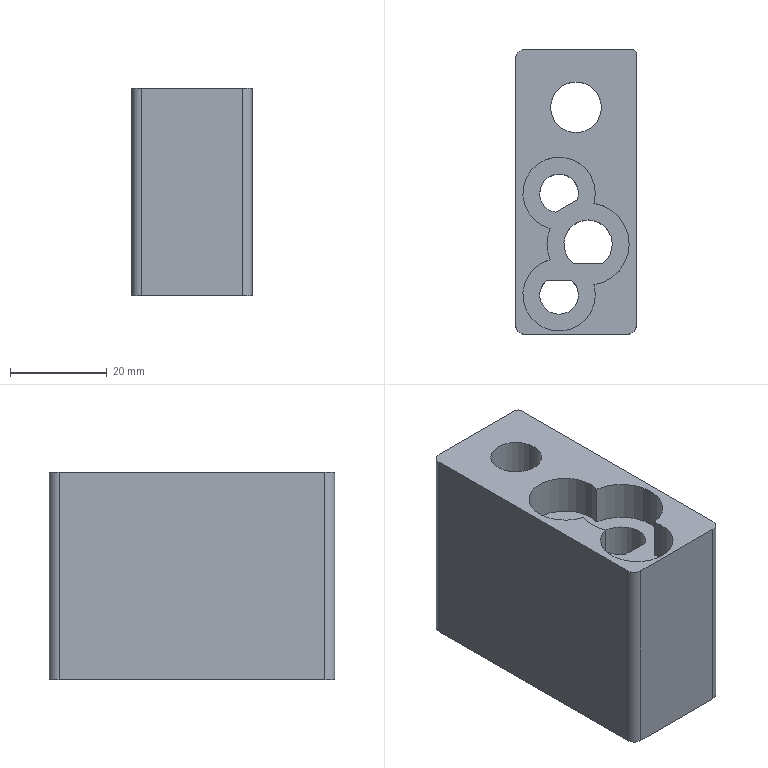Part | NX | features PH-16 2 | 1 solid | 26 faces | box 25 x 59 x 43 mm | volume 46890 mm3 | cylinder 14 | plane 12 | commonest cylinder face diameters 4 x3 8 x2 15 x2 17 x2 2 x1 6.001 x1
STEP:
#1=CARTESIAN_POINT('',(4127.236,-799.81,945.716));
#2=VERTEX_POINT('',#1);
#3=CARTESIAN_POINT('',(4127.236,-855.81,945.716));
#4=VERTEX_POINT('',#3);
#5=CARTESIAN_POINT('',(4127.236,-828.81,945.716));
#6=DIRECTION('',(0.,1.,0.));
#7=VECTOR('',#6,1000.);
#8=LINE('',#5,#7);
#9=EDGE_CURVE('',#2,#4,#8,.F.);
#10=ORIENTED_EDGE('',*,*,#9,.T.);
#11=CARTESIAN_POINT('',(4127.236,-855.81,902.716));
#12=VERTEX_POINT('',#11);
#13=CARTESIAN_POINT('',(4127.236,-855.81,915.716));
#14=DIRECTION('',(0.,0.,1.));
#15=VECTOR('',#14,1000.);
#16=LINE('',#13,#15);
#17=EDGE_CURVE('',#12,#4,#16,.T.);
#18=ORIENTED_EDGE('',*,*,#17,.F.);
#19=CARTESIAN_POINT('',(4127.236,-799.81,902.716));
#20=VERTEX_POINT('',#19);
#21=CARTESIAN_POINT('',(4127.236,-828.81,902.716));
#22=DIRECTION('',(0.,-1.,0.));
#23=VECTOR('',#22,1000.);
#24=LINE('',#21,#23);
#25=EDGE_CURVE('',#20,#12,#24,.T.);
#26=ORIENTED_EDGE('',*,*,#25,.F.);
#27=CARTESIAN_POINT('',(4127.236,-799.81,915.716));
#28=DIRECTION('',(0.,0.,1.));
#29=VECTOR('',#28,1000.);
#30=LINE('',#27,#29);
#31=EDGE_CURVE('',#2,#20,#30,.F.);
#32=ORIENTED_EDGE('',*,*,#31,.F.);
#33=EDGE_LOOP('',(#10,#18,#26,#32));
#34=FACE_BOUND('',#33,.T.);
#35=CARTESIAN_POINT('',(4127.236,-828.81,915.716));
#36=DIRECTION('',(1.,0.,0.));
#37=DIRECTION('',(0.,0.,1.));
#38=AXIS2_PLACEMENT_3D('',#35,#36,#37);
#39=PLANE('',#38);
#40=ADVANCED_FACE('',(#34),#39,.T.);
#41=CARTESIAN_POINT('',(4126.236,-798.81,902.716));
#42=VERTEX_POINT('',#41);
#43=CARTESIAN_POINT('',(4126.236,-799.81,902.716));
#44=DIRECTION('',(0.,0.,-1.));
#45=DIRECTION('',(-1.,0.,0.));
#46=AXIS2_PLACEMENT_3D('',#43,#44,#45);
#47=CIRCLE('',#46,1.);
#48=EDGE_CURVE('',#20,#42,#47,.F.);
#49=ORIENTED_EDGE('',*,*,#48,.T.);
#50=CARTESIAN_POINT('',(4126.236,-798.81,945.716));
#51=VERTEX_POINT('',#50);
#52=CARTESIAN_POINT('',(4126.236,-798.81,915.716));
#53=DIRECTION('',(0.,0.,1.));
#54=VECTOR('',#53,1000.);
#55=LINE('',#52,#54);
#56=EDGE_CURVE('',#42,#51,#55,.T.);
#57=ORIENTED_EDGE('',*,*,#56,.T.);
#58=CARTESIAN_POINT('',(4126.236,-799.81,945.716));
#59=DIRECTION('',(0.,0.,-1.));
#60=DIRECTION('',(1.,0.,0.));
#61=AXIS2_PLACEMENT_3D('',#58,#59,#60);
#62=CIRCLE('',#61,1.);
#63=EDGE_CURVE('',#51,#2,#62,.T.);
#64=ORIENTED_EDGE('',*,*,#63,.T.);
#65=ORIENTED_EDGE('',*,*,#31,.T.);
#66=EDGE_LOOP('',(#49,#57,#64,#65));
#67=FACE_BOUND('',#66,.T.);
#68=CARTESIAN_POINT('',(4126.236,-799.81,915.716));
#69=DIRECTION('',(0.,0.,1.));
#70=DIRECTION('',(1.,0.,0.));
#71=AXIS2_PLACEMENT_3D('',#68,#69,#70);
#72=CYLINDRICAL_SURFACE('',#71,1.);
#73=ADVANCED_FACE('',(#67),#72,.T.);
#74=CARTESIAN_POINT('',(4125.236,-857.81,902.716));
#75=VERTEX_POINT('',#74);
#76=CARTESIAN_POINT('',(4104.236,-857.81,902.716));
#77=VERTEX_POINT('',#76);
#78=CARTESIAN_POINT('',(4114.736,-857.81,902.716));
#79=DIRECTION('',(-1.,0.,0.));
#80=VECTOR('',#79,1000.);
#81=LINE('',#78,#80);
#82=EDGE_CURVE('',#75,#77,#81,.T.);
#83=ORIENTED_EDGE('',*,*,#82,.F.);
#84=CARTESIAN_POINT('',(4125.236,-857.81,945.716));
#85=VERTEX_POINT('',#84);
#86=CARTESIAN_POINT('',(4125.236,-857.81,915.716));
#87=DIRECTION('',(0.,0.,1.));
#88=VECTOR('',#87,1000.);
#89=LINE('',#86,#88);
#90=EDGE_CURVE('',#85,#75,#89,.F.);
#91=ORIENTED_EDGE('',*,*,#90,.F.);
#92=CARTESIAN_POINT('',(4104.236,-857.81,945.716));
#93=VERTEX_POINT('',#92);
#94=CARTESIAN_POINT('',(4114.736,-857.81,945.716));
#95=DIRECTION('',(1.,0.,0.));
#96=VECTOR('',#95,1000.);
#97=LINE('',#94,#96);
#98=EDGE_CURVE('',#85,#93,#97,.F.);
#99=ORIENTED_EDGE('',*,*,#98,.T.);
#100=CARTESIAN_POINT('',(4104.236,-857.81,915.716));
#101=DIRECTION('',(0.,0.,1.));
#102=VECTOR('',#101,1000.);
#103=LINE('',#100,#102);
#104=EDGE_CURVE('',#77,#93,#103,.T.);
#105=ORIENTED_EDGE('',*,*,#104,.F.);
#106=EDGE_LOOP('',(#83,#91,#99,#105));
#107=FACE_BOUND('',#106,.T.);
#108=CARTESIAN_POINT('',(4114.736,-857.81,915.716));
#109=DIRECTION('',(0.,-1.,0.));
#110=DIRECTION('',(0.,0.,-1.));
#111=AXIS2_PLACEMENT_3D('',#108,#109,#110);
#112=PLANE('',#111);
#113=ADVANCED_FACE('',(#107),#112,.T.);
#114=CARTESIAN_POINT('',(4125.236,-855.81,902.716));
#115=DIRECTION('',(0.,0.,-1.));
#116=DIRECTION('',(-1.,0.,0.));
#117=AXIS2_PLACEMENT_3D('',#114,#115,#116);
#118=CIRCLE('',#117,2.);
#119=EDGE_CURVE('',#75,#12,#118,.F.);
#120=ORIENTED_EDGE('',*,*,#119,.T.);
#121=ORIENTED_EDGE('',*,*,#17,.T.);
#122=CARTESIAN_POINT('',(4125.236,-855.81,945.716));
#123=DIRECTION('',(0.,0.,-1.));
#124=DIRECTION('',(1.,0.,0.));
#125=AXIS2_PLACEMENT_3D('',#122,#123,#124);
#126=CIRCLE('',#125,2.);
#127=EDGE_CURVE('',#4,#85,#126,.T.);
#128=ORIENTED_EDGE('',*,*,#127,.T.);
#129=ORIENTED_EDGE('',*,*,#90,.T.);
#130=EDGE_LOOP('',(#120,#121,#128,#129));
#131=FACE_BOUND('',#130,.T.);
#132=CARTESIAN_POINT('',(4125.236,-855.81,915.716));
#133=DIRECTION('',(0.,0.,1.));
#134=DIRECTION('',(1.,0.,0.));
#135=AXIS2_PLACEMENT_3D('',#132,#133,#134);
#136=CYLINDRICAL_SURFACE('',#135,2.);
#137=ADVANCED_FACE('',(#131),#136,.T.);
#138=CARTESIAN_POINT('',(4104.236,-798.81,902.716));
#139=VERTEX_POINT('',#138);
#140=CARTESIAN_POINT('',(4114.736,-798.81,902.716));
#141=DIRECTION('',(1.,0.,0.));
#142=VECTOR('',#141,1000.);
#143=LINE('',#140,#142);
#144=EDGE_CURVE('',#42,#139,#143,.F.);
#145=ORIENTED_EDGE('',*,*,#144,.T.);
#146=CARTESIAN_POINT('',(4104.236,-798.81,945.716));
#147=VERTEX_POINT('',#146);
#148=CARTESIAN_POINT('',(4104.236,-798.81,915.716));
#149=DIRECTION('',(0.,0.,1.));
#150=VECTOR('',#149,1000.);
#151=LINE('',#148,#150);
#152=EDGE_CURVE('',#147,#139,#151,.F.);
#153=ORIENTED_EDGE('',*,*,#152,.F.);
#154=CARTESIAN_POINT('',(4114.736,-798.81,945.716));
#155=DIRECTION('',(-1.,0.,0.));
#156=VECTOR('',#155,1000.);
#157=LINE('',#154,#156);
#158=EDGE_CURVE('',#147,#51,#157,.F.);
#159=ORIENTED_EDGE('',*,*,#158,.T.);
#160=ORIENTED_EDGE('',*,*,#56,.F.);
#161=EDGE_LOOP('',(#145,#153,#159,#160));
#162=FACE_BOUND('',#161,.T.);
#163=CARTESIAN_POINT('',(4114.736,-798.81,915.716));
#164=DIRECTION('',(0.,1.,0.));
#165=DIRECTION('',(0.,0.,1.));
#166=AXIS2_PLACEMENT_3D('',#163,#164,#165);
#167=PLANE('',#166);
#168=ADVANCED_FACE('',(#162),#167,.T.);
#169=CARTESIAN_POINT('',(4102.236,-800.81,902.716));
#170=VERTEX_POINT('',#169);
#171=CARTESIAN_POINT('',(4102.236,-855.81,902.716));
#172=VERTEX_POINT('',#171);
#173=CARTESIAN_POINT('',(4102.236,-828.81,902.716));
#174=DIRECTION('',(0.,1.,0.));
#175=VECTOR('',#174,1000.);
#176=LINE('',#173,#175);
#177=EDGE_CURVE('',#170,#172,#176,.F.);
#178=ORIENTED_EDGE('',*,*,#177,.T.);
#179=CARTESIAN_POINT('',(4102.236,-855.81,945.716));
#180=VERTEX_POINT('',#179);
#181=CARTESIAN_POINT('',(4102.236,-855.81,915.716));
#182=DIRECTION('',(0.,0.,1.));
#183=VECTOR('',#182,1000.);
#184=LINE('',#181,#183);
#185=EDGE_CURVE('',#180,#172,#184,.F.);
#186=ORIENTED_EDGE('',*,*,#185,.F.);
#187=CARTESIAN_POINT('',(4102.236,-800.81,945.716));
#188=VERTEX_POINT('',#187);
#189=CARTESIAN_POINT('',(4102.236,-828.81,945.716));
#190=DIRECTION('',(0.,-1.,0.));
#191=VECTOR('',#190,1000.);
#192=LINE('',#189,#191);
#193=EDGE_CURVE('',#180,#188,#192,.F.);
#194=ORIENTED_EDGE('',*,*,#193,.T.);
#195=CARTESIAN_POINT('',(4102.236,-800.81,915.716));
#196=DIRECTION('',(0.,0.,1.));
#197=VECTOR('',#196,1000.);
#198=LINE('',#195,#197);
#199=EDGE_CURVE('',#170,#188,#198,.T.);
#200=ORIENTED_EDGE('',*,*,#199,.F.);
#201=EDGE_LOOP('',(#178,#186,#194,#200));
#202=FACE_BOUND('',#201,.T.);
#203=CARTESIAN_POINT('',(4102.236,-828.81,915.716));
#204=DIRECTION('',(-1.,0.,0.));
#205=DIRECTION('',(0.,0.,-1.));
#206=AXIS2_PLACEMENT_3D('',#203,#204,#205);
#207=PLANE('',#206);
#208=ADVANCED_FACE('',(#202),#207,.T.);
#209=CARTESIAN_POINT('',(4104.236,-855.81,902.716));
#210=DIRECTION('',(0.,0.,-1.));
#211=DIRECTION('',(-1.,0.,0.));
#212=AXIS2_PLACEMENT_3D('',#209,#210,#211);
#213=CIRCLE('',#212,2.);
#214=EDGE_CURVE('',#172,#77,#213,.F.);
#215=ORIENTED_EDGE('',*,*,#214,.T.);
#216=ORIENTED_EDGE('',*,*,#104,.T.);
#217=CARTESIAN_POINT('',(4104.236,-855.81,945.716));
#218=DIRECTION('',(0.,0.,-1.));
#219=DIRECTION('',(1.,0.,0.));
#220=AXIS2_PLACEMENT_3D('',#217,#218,#219);
#221=CIRCLE('',#220,2.);
#222=EDGE_CURVE('',#93,#180,#221,.T.);
#223=ORIENTED_EDGE('',*,*,#222,.T.);
#224=ORIENTED_EDGE('',*,*,#185,.T.);
#225=EDGE_LOOP('',(#215,#216,#223,#224));
#226=FACE_BOUND('',#225,.T.);
#227=CARTESIAN_POINT('',(4104.236,-855.81,915.716));
#228=DIRECTION('',(0.,0.,1.));
#229=DIRECTION('',(1.,0.,0.));
#230=AXIS2_PLACEMENT_3D('',#227,#228,#229);
#231=CYLINDRICAL_SURFACE('',#230,2.);
#232=ADVANCED_FACE('',(#226),#231,.T.);
#233=CARTESIAN_POINT('',(4104.236,-800.81,902.716));
#234=DIRECTION('',(0.,0.,-1.));
#235=DIRECTION('',(-1.,0.,0.));
#236=AXIS2_PLACEMENT_3D('',#233,#234,#235);
#237=CIRCLE('',#236,2.);
#238=EDGE_CURVE('',#139,#170,#237,.F.);
#239=ORIENTED_EDGE('',*,*,#238,.T.);
#240=ORIENTED_EDGE('',*,*,#199,.T.);
#241=CARTESIAN_POINT('',(4104.236,-800.81,945.716));
#242=DIRECTION('',(0.,0.,-1.));
#243=DIRECTION('',(1.,0.,0.));
#244=AXIS2_PLACEMENT_3D('',#241,#242,#243);
#245=CIRCLE('',#244,2.);
#246=EDGE_CURVE('',#188,#147,#245,.T.);
#247=ORIENTED_EDGE('',*,*,#246,.T.);
#248=ORIENTED_EDGE('',*,*,#152,.T.);
#249=EDGE_LOOP('',(#239,#240,#247,#248));
#250=FACE_BOUND('',#249,.T.);
#251=CARTESIAN_POINT('',(4104.236,-800.81,915.716));
#252=DIRECTION('',(0.,0.,1.));
#253=DIRECTION('',(1.,0.,0.));
#254=AXIS2_PLACEMENT_3D('',#251,#252,#253);
#255=CYLINDRICAL_SURFACE('',#254,2.);
#256=ADVANCED_FACE('',(#250),#255,.T.);
#257=CARTESIAN_POINT('',(4110.445,-832.543,937.416));
#258=VERTEX_POINT('',#257);
#259=CARTESIAN_POINT('',(4110.445,-832.543,902.716));
#260=VERTEX_POINT('',#259);
#261=CARTESIAN_POINT('',(4110.445,-832.543,940.716));
#262=DIRECTION('',(0.,0.,-1.));
#263=VECTOR('',#262,1000.);
#264=LINE('',#261,#263);
#265=EDGE_CURVE('',#258,#260,#264,.T.);
#266=ORIENTED_EDGE('',*,*,#265,.F.);
#267=CARTESIAN_POINT('',(4115.028,-829.898,937.416));
#268=VERTEX_POINT('',#267);
#269=CARTESIAN_POINT('',(4103.643,-836.471,937.416));
#270=DIRECTION('',(0.866,0.5,0.));
#271=VECTOR('',#270,1000.);
#272=LINE('',#269,#271);
#273=EDGE_CURVE('',#258,#268,#272,.T.);
#274=ORIENTED_EDGE('',*,*,#273,.T.);
#275=CARTESIAN_POINT('',(4115.028,-829.898,902.716));
#276=VERTEX_POINT('',#275);
#277=CARTESIAN_POINT('',(4115.028,-829.898,940.716));
#278=DIRECTION('',(0.,0.,-1.));
#279=VECTOR('',#278,1000.);
#280=LINE('',#277,#279);
#281=EDGE_CURVE('',#276,#268,#280,.F.);
#282=ORIENTED_EDGE('',*,*,#281,.F.);
#283=CARTESIAN_POINT('',(4109.15,-833.291,902.716));
#284=DIRECTION('',(0.866,0.5,0.));
#285=VECTOR('',#284,1000.);
#286=LINE('',#283,#285);
#287=EDGE_CURVE('',#260,#276,#286,.T.);
#288=ORIENTED_EDGE('',*,*,#287,.F.);
#289=EDGE_LOOP('',(#266,#274,#282,#288));
#290=FACE_BOUND('',#289,.T.);
#291=CARTESIAN_POINT('',(4106.744,-834.68,940.716));
#292=DIRECTION('',(-0.5,0.866,0.));
#293=DIRECTION('',(0.866,0.5,0.));
#294=AXIS2_PLACEMENT_3D('',#291,#292,#293);
#295=PLANE('',#294);
#296=ADVANCED_FACE('',(#290),#295,.T.);
#297=CARTESIAN_POINT('',(4111.236,-828.623,902.716));
#298=DIRECTION('',(0.,0.,-1.));
#299=DIRECTION('',(-1.,0.,0.));
#300=AXIS2_PLACEMENT_3D('',#297,#298,#299);
#301=CIRCLE('',#300,4.);
#302=EDGE_CURVE('',#260,#276,#301,.T.);
#303=ORIENTED_EDGE('',*,*,#302,.T.);
#304=ORIENTED_EDGE('',*,*,#281,.T.);
#305=CARTESIAN_POINT('',(4111.236,-828.623,937.416));
#306=DIRECTION('',(0.,0.,-1.));
#307=DIRECTION('',(-1.,0.,0.));
#308=AXIS2_PLACEMENT_3D('',#305,#306,#307);
#309=CIRCLE('',#308,4.);
#310=EDGE_CURVE('',#258,#268,#309,.T.);
#311=ORIENTED_EDGE('',*,*,#310,.F.);
#312=ORIENTED_EDGE('',*,*,#265,.T.);
#313=EDGE_LOOP('',(#303,#304,#311,#312));
#314=FACE_BOUND('',#313,.T.);
#315=CARTESIAN_POINT('',(4111.236,-828.623,940.716));
#316=DIRECTION('',(0.,0.,-1.));
#317=DIRECTION('',(-0.866,-0.5,0.));
#318=AXIS2_PLACEMENT_3D('',#315,#316,#317);
#319=CYLINDRICAL_SURFACE('',#318,4.);
#320=ADVANCED_FACE('',(#314),#319,.F.);
#321=CARTESIAN_POINT('',(4120.236,-843.122,902.716));
#322=VERTEX_POINT('',#321);
#323=CARTESIAN_POINT('',(4114.236,-843.122,902.716));
#324=VERTEX_POINT('',#323);
#325=CARTESIAN_POINT('',(4123.486,-843.122,902.716));
#326=DIRECTION('',(-1.,0.,0.));
#327=VECTOR('',#326,1000.);
#328=LINE('',#325,#327);
#329=EDGE_CURVE('',#322,#324,#328,.T.);
#330=ORIENTED_EDGE('',*,*,#329,.T.);
#331=CARTESIAN_POINT('',(4114.236,-843.122,937.416));
#332=VERTEX_POINT('',#331);
#333=CARTESIAN_POINT('',(4114.236,-843.122,881.498));
#334=DIRECTION('',(0.,0.,1.));
#335=VECTOR('',#334,1000.);
#336=LINE('',#333,#335);
#337=EDGE_CURVE('',#332,#324,#336,.F.);
#338=ORIENTED_EDGE('',*,*,#337,.F.);
#339=CARTESIAN_POINT('',(4120.236,-843.122,937.416));
#340=VERTEX_POINT('',#339);
#341=CARTESIAN_POINT('',(4111.236,-843.122,937.416));
#342=DIRECTION('',(-1.,0.,0.));
#343=VECTOR('',#342,1000.);
#344=LINE('',#341,#343);
#345=EDGE_CURVE('',#340,#332,#344,.T.);
#346=ORIENTED_EDGE('',*,*,#345,.F.);
#347=CARTESIAN_POINT('',(4120.236,-843.122,936.216));
#348=DIRECTION('',(0.,0.,-1.));
#349=VECTOR('',#348,1000.);
#350=LINE('',#347,#349);
#351=EDGE_CURVE('',#322,#340,#350,.F.);
#352=ORIENTED_EDGE('',*,*,#351,.F.);
#353=EDGE_LOOP('',(#330,#338,#346,#352));
#354=FACE_BOUND('',#353,.T.);
#355=CARTESIAN_POINT('',(4124.849,-843.122,952.222));
#356=DIRECTION('',(0.,-1.,0.));
#357=DIRECTION('',(-1.,0.,0.));
#358=AXIS2_PLACEMENT_3D('',#355,#356,#357);
#359=PLANE('',#358);
#360=ADVANCED_FACE('',(#354),#359,.F.);
#361=CARTESIAN_POINT('',(4117.236,-839.122,902.716));
#362=DIRECTION('',(0.,0.,-1.));
#363=DIRECTION('',(-1.,0.,0.));
#364=AXIS2_PLACEMENT_3D('',#361,#362,#363);
#365=CIRCLE('',#364,5.);
#366=EDGE_CURVE('',#324,#322,#365,.T.);
#367=ORIENTED_EDGE('',*,*,#366,.T.);
#368=ORIENTED_EDGE('',*,*,#351,.T.);
#369=CARTESIAN_POINT('',(4117.236,-839.122,937.416));
#370=DIRECTION('',(0.,0.,-1.));
#371=DIRECTION('',(-1.,0.,0.));
#372=AXIS2_PLACEMENT_3D('',#369,#370,#371);
#373=CIRCLE('',#372,5.);
#374=EDGE_CURVE('',#332,#340,#373,.T.);
#375=ORIENTED_EDGE('',*,*,#374,.F.);
#376=ORIENTED_EDGE('',*,*,#337,.T.);
#377=EDGE_LOOP('',(#367,#368,#375,#376));
#378=FACE_BOUND('',#377,.T.);
#379=CARTESIAN_POINT('',(4117.236,-839.122,906.216));
#380=DIRECTION('',(0.,0.,-1.));
#381=DIRECTION('',(0.008727,-1.,0.));
#382=AXIS2_PLACEMENT_3D('',#379,#380,#381);
#383=CYLINDRICAL_SURFACE('',#382,5.);
#384=ADVANCED_FACE('',(#378),#383,.F.);
#385=CARTESIAN_POINT('',(4111.187,-846.622,902.716));
#386=VERTEX_POINT('',#385);
#387=CARTESIAN_POINT('',(4111.187,-846.622,937.416));
#388=VERTEX_POINT('',#387);
#389=CARTESIAN_POINT('',(4111.187,-846.622,945.716));
#390=DIRECTION('',(0.,0.,-1.));
#391=VECTOR('',#390,1000.);
#392=LINE('',#389,#391);
#393=EDGE_CURVE('',#386,#388,#392,.F.);
#394=ORIENTED_EDGE('',*,*,#393,.T.);
#395=CARTESIAN_POINT('',(4108.59,-846.622,937.416));
#396=VERTEX_POINT('',#395);
#397=CARTESIAN_POINT('',(4111.236,-846.622,937.416));
#398=DIRECTION('',(-1.,0.,0.));
#399=VECTOR('',#398,1000.);
#400=LINE('',#397,#399);
#401=EDGE_CURVE('',#388,#396,#400,.T.);
#402=ORIENTED_EDGE('',*,*,#401,.T.);
#403=CARTESIAN_POINT('',(4108.59,-846.622,902.716));
#404=VERTEX_POINT('',#403);
#405=CARTESIAN_POINT('',(4108.59,-846.622,940.716));
#406=DIRECTION('',(0.,0.,-1.));
#407=VECTOR('',#406,1000.);
#408=LINE('',#405,#407);
#409=EDGE_CURVE('',#396,#404,#408,.T.);
#410=ORIENTED_EDGE('',*,*,#409,.T.);
#411=CARTESIAN_POINT('',(4123.486,-846.622,902.716));
#412=DIRECTION('',(-1.,0.,0.));
#413=VECTOR('',#412,1000.);
#414=LINE('',#411,#413);
#415=EDGE_CURVE('',#386,#404,#414,.T.);
#416=ORIENTED_EDGE('',*,*,#415,.F.);
#417=EDGE_LOOP('',(#394,#402,#410,#416));
#418=FACE_BOUND('',#417,.T.);
#419=CARTESIAN_POINT('',(4104.317,-846.622,940.716));
#420=DIRECTION('',(0.,-1.,0.));
#421=DIRECTION('',(1.,0.,0.));
#422=AXIS2_PLACEMENT_3D('',#419,#420,#421);
#423=PLANE('',#422);
#424=ADVANCED_FACE('',(#418),#423,.T.);
#425=ORIENTED_EDGE('',*,*,#393,.F.);
#426=CARTESIAN_POINT('',(4111.285,-846.622,902.716));
#427=VERTEX_POINT('',#426);
#428=CARTESIAN_POINT('',(4111.236,-849.622,902.716));
#429=DIRECTION('',(0.,0.,-1.));
#430=DIRECTION('',(-1.,0.,0.));
#431=AXIS2_PLACEMENT_3D('',#428,#429,#430);
#432=CIRCLE('',#431,3.);
#433=EDGE_CURVE('',#386,#427,#432,.T.);
#434=ORIENTED_EDGE('',*,*,#433,.T.);
#435=CARTESIAN_POINT('',(4111.285,-846.622,937.416));
#436=VERTEX_POINT('',#435);
#437=CARTESIAN_POINT('',(4111.285,-846.622,945.716));
#438=DIRECTION('',(0.,0.,-1.));
#439=VECTOR('',#438,1000.);
#440=LINE('',#437,#439);
#441=EDGE_CURVE('',#436,#427,#440,.T.);
#442=ORIENTED_EDGE('',*,*,#441,.F.);
#443=CARTESIAN_POINT('',(4111.236,-849.622,937.416));
#444=DIRECTION('',(0.,0.,-1.));
#445=DIRECTION('',(-1.,0.,0.));
#446=AXIS2_PLACEMENT_3D('',#443,#444,#445);
#447=CIRCLE('',#446,3.);
#448=EDGE_CURVE('',#388,#436,#447,.T.);
#449=ORIENTED_EDGE('',*,*,#448,.F.);
#450=EDGE_LOOP('',(#425,#434,#442,#449));
#451=FACE_BOUND('',#450,.T.);
#452=CARTESIAN_POINT('',(4111.236,-849.622,945.716));
#453=DIRECTION('',(0.,0.,-1.));
#454=DIRECTION('',(1.,0.,0.));
#455=AXIS2_PLACEMENT_3D('',#452,#453,#454);
#456=CYLINDRICAL_SURFACE('',#455,3.);
#457=ADVANCED_FACE('',(#451),#456,.F.);
#458=CARTESIAN_POINT('',(4113.882,-846.622,902.716));
#459=VERTEX_POINT('',#458);
#460=CARTESIAN_POINT('',(4113.882,-846.622,937.416));
#461=VERTEX_POINT('',#460);
#462=CARTESIAN_POINT('',(4113.882,-846.622,940.716));
#463=DIRECTION('',(0.,0.,-1.));
#464=VECTOR('',#463,1000.);
#465=LINE('',#462,#464);
#466=EDGE_CURVE('',#459,#461,#465,.F.);
#467=ORIENTED_EDGE('',*,*,#466,.T.);
#468=CARTESIAN_POINT('',(4111.236,-846.622,937.416));
#469=DIRECTION('',(-1.,0.,0.));
#470=VECTOR('',#469,1000.);
#471=LINE('',#468,#470);
#472=EDGE_CURVE('',#461,#436,#471,.T.);
#473=ORIENTED_EDGE('',*,*,#472,.T.);
#474=ORIENTED_EDGE('',*,*,#441,.T.);
#475=CARTESIAN_POINT('',(4123.486,-846.622,902.716));
#476=DIRECTION('',(-1.,0.,0.));
#477=VECTOR('',#476,1000.);
#478=LINE('',#475,#477);
#479=EDGE_CURVE('',#459,#427,#478,.T.);
#480=ORIENTED_EDGE('',*,*,#479,.F.);
#481=EDGE_LOOP('',(#467,#473,#474,#480));
#482=FACE_BOUND('',#481,.T.);
#483=CARTESIAN_POINT('',(4104.317,-846.622,940.716));
#484=DIRECTION('',(0.,-1.,0.));
#485=DIRECTION('',(1.,0.,0.));
#486=AXIS2_PLACEMENT_3D('',#483,#484,#485);
#487=PLANE('',#486);
#488=ADVANCED_FACE('',(#482),#487,.T.);
#489=CARTESIAN_POINT('',(4111.236,-849.622,902.716));
#490=DIRECTION('',(0.,0.,-1.));
#491=DIRECTION('',(-1.,0.,0.));
#492=AXIS2_PLACEMENT_3D('',#489,#490,#491);
#493=CIRCLE('',#492,4.);
#494=EDGE_CURVE('',#459,#404,#493,.T.);
#495=ORIENTED_EDGE('',*,*,#494,.T.);
#496=ORIENTED_EDGE('',*,*,#409,.F.);
#497=CARTESIAN_POINT('',(4111.236,-849.622,937.416));
#498=DIRECTION('',(0.,0.,-1.));
#499=DIRECTION('',(-1.,0.,0.));
#500=AXIS2_PLACEMENT_3D('',#497,#498,#499);
#501=CIRCLE('',#500,4.);
#502=EDGE_CURVE('',#461,#396,#501,.T.);
#503=ORIENTED_EDGE('',*,*,#502,.F.);
#504=ORIENTED_EDGE('',*,*,#466,.F.);
#505=EDGE_LOOP('',(#495,#496,#503,#504));
#506=FACE_BOUND('',#505,.T.);
#507=CARTESIAN_POINT('',(4111.236,-849.622,940.716));
#508=DIRECTION('',(0.,0.,-1.));
#509=DIRECTION('',(-1.,0.,0.));
#510=AXIS2_PLACEMENT_3D('',#507,#508,#509);
#511=CYLINDRICAL_SURFACE('',#510,4.);
#512=ADVANCED_FACE('',(#506),#511,.F.);
#513=CARTESIAN_POINT('',(4123.736,-810.81,902.716));
#514=VERTEX_POINT('',#513);
#515=CARTESIAN_POINT('',(4114.736,-810.81,902.716));
#516=DIRECTION('',(0.,0.,1.));
#517=DIRECTION('',(1.,0.,0.));
#518=AXIS2_PLACEMENT_3D('',#515,#516,#517);
#519=CIRCLE('',#518,9.);
#520=EDGE_CURVE('',#514,#514,#519,.T.);
#521=ORIENTED_EDGE('',*,*,#520,.T.);
#522=EDGE_LOOP('',(#521));
#523=FACE_BOUND('',#522,.T.);
#524=ORIENTED_EDGE('',*,*,#494,.F.);
#525=ORIENTED_EDGE('',*,*,#479,.T.);
#526=ORIENTED_EDGE('',*,*,#433,.F.);
#527=ORIENTED_EDGE('',*,*,#415,.T.);
#528=EDGE_LOOP('',(#524,#525,#526,#527));
#529=FACE_BOUND('',#528,.T.);
#530=ORIENTED_EDGE('',*,*,#366,.F.);
#531=ORIENTED_EDGE('',*,*,#329,.F.);
#532=EDGE_LOOP('',(#530,#531));
#533=FACE_BOUND('',#532,.T.);
#534=ORIENTED_EDGE('',*,*,#302,.F.);
#535=ORIENTED_EDGE('',*,*,#287,.T.);
#536=EDGE_LOOP('',(#534,#535));
#537=FACE_BOUND('',#536,.T.);
#538=ORIENTED_EDGE('',*,*,#25,.T.);
#539=ORIENTED_EDGE('',*,*,#119,.F.);
#540=ORIENTED_EDGE('',*,*,#82,.T.);
#541=ORIENTED_EDGE('',*,*,#214,.F.);
#542=ORIENTED_EDGE('',*,*,#177,.F.);
#543=ORIENTED_EDGE('',*,*,#238,.F.);
#544=ORIENTED_EDGE('',*,*,#144,.F.);
#545=ORIENTED_EDGE('',*,*,#48,.F.);
#546=EDGE_LOOP('',(#538,#539,#540,#541,#542,#543,#544,#545));
#547=FACE_BOUND('',#546,.T.);
#548=CARTESIAN_POINT('',(4123.486,-858.122,902.716));
#549=DIRECTION('',(0.,0.,-1.));
#550=DIRECTION('',(-1.,0.,0.));
#551=AXIS2_PLACEMENT_3D('',#548,#549,#550);
#552=PLANE('',#551);
#553=ADVANCED_FACE('',(#523,#529,#533,#537,#547),#552,.T.);
#554=ORIENTED_EDGE('',*,*,#273,.F.);
#555=ORIENTED_EDGE('',*,*,#310,.T.);
#556=EDGE_LOOP('',(#554,#555));
#557=FACE_BOUND('',#556,.T.);
#558=CARTESIAN_POINT('',(4109.376,-835.888,937.416));
#559=VERTEX_POINT('',#558);
#560=CARTESIAN_POINT('',(4109.375,-842.357,937.416));
#561=VERTEX_POINT('',#560);
#562=CARTESIAN_POINT('',(4117.236,-839.122,937.416));
#563=DIRECTION('',(0.,0.,1.));
#564=DIRECTION('',(1.,0.,0.));
#565=AXIS2_PLACEMENT_3D('',#562,#563,#564);
#566=CIRCLE('',#565,8.5);
#567=EDGE_CURVE('',#559,#561,#566,.T.);
#568=ORIENTED_EDGE('',*,*,#567,.T.);
#569=CARTESIAN_POINT('',(4118.44,-847.536,937.416));
#570=VERTEX_POINT('',#569);
#571=CARTESIAN_POINT('',(4111.236,-849.622,937.416));
#572=DIRECTION('',(0.,0.,1.));
#573=DIRECTION('',(1.,0.,0.));
#574=AXIS2_PLACEMENT_3D('',#571,#572,#573);
#575=CIRCLE('',#574,7.5);
#576=EDGE_CURVE('',#561,#570,#575,.T.);
#577=ORIENTED_EDGE('',*,*,#576,.T.);
#578=CARTESIAN_POINT('',(4118.44,-830.708,937.416));
#579=VERTEX_POINT('',#578);
#580=CARTESIAN_POINT('',(4117.236,-839.122,937.416));
#581=DIRECTION('',(0.,0.,1.));
#582=DIRECTION('',(1.,0.,0.));
#583=AXIS2_PLACEMENT_3D('',#580,#581,#582);
#584=CIRCLE('',#583,8.5);
#585=EDGE_CURVE('',#570,#579,#584,.T.);
#586=ORIENTED_EDGE('',*,*,#585,.T.);
#587=CARTESIAN_POINT('',(4111.236,-828.622,937.416));
#588=DIRECTION('',(0.,0.,1.));
#589=DIRECTION('',(1.,0.,0.));
#590=AXIS2_PLACEMENT_3D('',#587,#588,#589);
#591=CIRCLE('',#590,7.5);
#592=EDGE_CURVE('',#579,#559,#591,.T.);
#593=ORIENTED_EDGE('',*,*,#592,.T.);
#594=EDGE_LOOP('',(#568,#577,#586,#593));
#595=FACE_BOUND('',#594,.T.);
#596=ORIENTED_EDGE('',*,*,#345,.T.);
#597=ORIENTED_EDGE('',*,*,#374,.T.);
#598=EDGE_LOOP('',(#596,#597));
#599=FACE_BOUND('',#598,.T.);
#600=ORIENTED_EDGE('',*,*,#472,.F.);
#601=ORIENTED_EDGE('',*,*,#502,.T.);
#602=ORIENTED_EDGE('',*,*,#401,.F.);
#603=ORIENTED_EDGE('',*,*,#448,.T.);
#604=EDGE_LOOP('',(#600,#601,#602,#603));
#605=FACE_BOUND('',#604,.T.);
#606=CARTESIAN_POINT('',(4111.236,-849.622,937.416));
#607=DIRECTION('',(0.,0.,-1.));
#608=DIRECTION('',(-1.,0.,0.));
#609=AXIS2_PLACEMENT_3D('',#606,#607,#608);
#610=PLANE('',#609);
#611=ADVANCED_FACE('',(#557,#595,#599,#605),#610,.F.);
#612=ORIENTED_EDGE('',*,*,#585,.F.);
#613=CARTESIAN_POINT('',(4118.44,-847.536,945.716));
#614=VERTEX_POINT('',#613);
#615=CARTESIAN_POINT('',(4118.44,-847.536,941.566));
#616=DIRECTION('',(0.,0.,-1.));
#617=VECTOR('',#616,1000.);
#618=LINE('',#615,#617);
#619=EDGE_CURVE('',#614,#570,#618,.T.);
#620=ORIENTED_EDGE('',*,*,#619,.F.);
#621=CARTESIAN_POINT('',(4118.44,-830.708,945.716));
#622=VERTEX_POINT('',#621);
#623=CARTESIAN_POINT('',(4117.236,-839.122,945.716));
#624=DIRECTION('',(0.,0.,-1.));
#625=DIRECTION('',(1.,0.,0.));
#626=AXIS2_PLACEMENT_3D('',#623,#624,#625);
#627=CIRCLE('',#626,8.5);
#628=EDGE_CURVE('',#622,#614,#627,.T.);
#629=ORIENTED_EDGE('',*,*,#628,.F.);
#630=CARTESIAN_POINT('',(4118.44,-830.708,941.566));
#631=DIRECTION('',(0.,0.,-1.));
#632=VECTOR('',#631,1000.);
#633=LINE('',#630,#632);
#634=EDGE_CURVE('',#579,#622,#633,.F.);
#635=ORIENTED_EDGE('',*,*,#634,.F.);
#636=EDGE_LOOP('',(#612,#620,#629,#635));
#637=FACE_BOUND('',#636,.T.);
#638=CARTESIAN_POINT('',(4117.236,-839.122,945.716));
#639=DIRECTION('',(0.,0.,-1.));
#640=DIRECTION('',(1.,0.,0.));
#641=AXIS2_PLACEMENT_3D('',#638,#639,#640);
#642=CYLINDRICAL_SURFACE('',#641,8.5);
#643=ADVANCED_FACE('',(#637),#642,.F.);
#644=CARTESIAN_POINT('',(4109.376,-835.888,945.716));
#645=VERTEX_POINT('',#644);
#646=CARTESIAN_POINT('',(4111.236,-828.622,945.716));
#647=DIRECTION('',(0.,0.,-1.));
#648=DIRECTION('',(1.,0.,0.));
#649=AXIS2_PLACEMENT_3D('',#646,#647,#648);
#650=CIRCLE('',#649,7.5);
#651=EDGE_CURVE('',#645,#622,#650,.T.);
#652=ORIENTED_EDGE('',*,*,#651,.F.);
#653=CARTESIAN_POINT('',(4109.376,-835.888,941.566));
#654=DIRECTION('',(0.,0.,-1.));
#655=VECTOR('',#654,1000.);
#656=LINE('',#653,#655);
#657=EDGE_CURVE('',#645,#559,#656,.T.);
#658=ORIENTED_EDGE('',*,*,#657,.T.);
#659=ORIENTED_EDGE('',*,*,#592,.F.);
#660=ORIENTED_EDGE('',*,*,#634,.T.);
#661=EDGE_LOOP('',(#652,#658,#659,#660));
#662=FACE_BOUND('',#661,.T.);
#663=CARTESIAN_POINT('',(4111.236,-828.622,945.716));
#664=DIRECTION('',(0.,0.,-1.));
#665=DIRECTION('',(1.,0.,0.));
#666=AXIS2_PLACEMENT_3D('',#663,#664,#665);
#667=CYLINDRICAL_SURFACE('',#666,7.5);
#668=ADVANCED_FACE('',(#662),#667,.F.);
#669=CARTESIAN_POINT('',(4109.375,-842.357,945.716));
#670=VERTEX_POINT('',#669);
#671=CARTESIAN_POINT('',(4117.236,-839.122,945.716));
#672=DIRECTION('',(0.,0.,-1.));
#673=DIRECTION('',(1.,0.,0.));
#674=AXIS2_PLACEMENT_3D('',#671,#672,#673);
#675=CIRCLE('',#674,8.5);
#676=EDGE_CURVE('',#670,#645,#675,.T.);
#677=ORIENTED_EDGE('',*,*,#676,.F.);
#678=CARTESIAN_POINT('',(4109.375,-842.357,941.566));
#679=DIRECTION('',(0.,0.,-1.));
#680=VECTOR('',#679,1000.);
#681=LINE('',#678,#680);
#682=EDGE_CURVE('',#561,#670,#681,.F.);
#683=ORIENTED_EDGE('',*,*,#682,.F.);
#684=ORIENTED_EDGE('',*,*,#567,.F.);
#685=ORIENTED_EDGE('',*,*,#657,.F.);
#686=EDGE_LOOP('',(#677,#683,#684,#685));
#687=FACE_BOUND('',#686,.T.);
#688=CARTESIAN_POINT('',(4117.236,-839.122,945.716));
#689=DIRECTION('',(0.,0.,-1.));
#690=DIRECTION('',(1.,0.,0.));
#691=AXIS2_PLACEMENT_3D('',#688,#689,#690);
#692=CYLINDRICAL_SURFACE('',#691,8.5);
#693=ADVANCED_FACE('',(#687),#692,.F.);
#694=CARTESIAN_POINT('',(4111.236,-849.622,945.716));
#695=DIRECTION('',(0.,0.,-1.));
#696=DIRECTION('',(1.,0.,0.));
#697=AXIS2_PLACEMENT_3D('',#694,#695,#696);
#698=CIRCLE('',#697,7.5);
#699=EDGE_CURVE('',#614,#670,#698,.T.);
#700=ORIENTED_EDGE('',*,*,#699,.F.);
#701=ORIENTED_EDGE('',*,*,#619,.T.);
#702=ORIENTED_EDGE('',*,*,#576,.F.);
#703=ORIENTED_EDGE('',*,*,#682,.T.);
#704=EDGE_LOOP('',(#700,#701,#702,#703));
#705=FACE_BOUND('',#704,.T.);
#706=CARTESIAN_POINT('',(4111.236,-849.622,945.716));
#707=DIRECTION('',(0.,0.,-1.));
#708=DIRECTION('',(1.,0.,0.));
#709=AXIS2_PLACEMENT_3D('',#706,#707,#708);
#710=CYLINDRICAL_SURFACE('',#709,7.5);
#711=ADVANCED_FACE('',(#705),#710,.F.);
#712=CARTESIAN_POINT('',(4119.986,-810.81,945.716));
#713=VERTEX_POINT('',#712);
#714=CARTESIAN_POINT('',(4114.736,-810.81,945.716));
#715=DIRECTION('',(0.,0.,1.));
#716=DIRECTION('',(1.,0.,0.));
#717=AXIS2_PLACEMENT_3D('',#714,#715,#716);
#718=CIRCLE('',#717,5.25);
#719=EDGE_CURVE('',#713,#713,#718,.T.);
#720=ORIENTED_EDGE('',*,*,#719,.F.);
#721=EDGE_LOOP('',(#720));
#722=FACE_BOUND('',#721,.T.);
#723=ORIENTED_EDGE('',*,*,#699,.T.);
#724=ORIENTED_EDGE('',*,*,#676,.T.);
#725=ORIENTED_EDGE('',*,*,#651,.T.);
#726=ORIENTED_EDGE('',*,*,#628,.T.);
#727=EDGE_LOOP('',(#723,#724,#725,#726));
#728=FACE_BOUND('',#727,.T.);
#729=ORIENTED_EDGE('',*,*,#98,.F.);
#730=ORIENTED_EDGE('',*,*,#127,.F.);
#731=ORIENTED_EDGE('',*,*,#9,.F.);
#732=ORIENTED_EDGE('',*,*,#63,.F.);
#733=ORIENTED_EDGE('',*,*,#158,.F.);
#734=ORIENTED_EDGE('',*,*,#246,.F.);
#735=ORIENTED_EDGE('',*,*,#193,.F.);
#736=ORIENTED_EDGE('',*,*,#222,.F.);
#737=EDGE_LOOP('',(#729,#730,#731,#732,#733,#734,#735,#736));
#738=FACE_BOUND('',#737,.T.);
#739=CARTESIAN_POINT('',(4123.486,-858.122,945.716));
#740=DIRECTION('',(0.,0.,1.));
#741=DIRECTION('',(1.,0.,0.));
#742=AXIS2_PLACEMENT_3D('',#739,#740,#741);
#743=PLANE('',#742);
#744=ADVANCED_FACE('',(#722,#728,#738),#743,.T.);
#745=ORIENTED_EDGE('',*,*,#719,.T.);
#746=EDGE_LOOP('',(#745));
#747=FACE_BOUND('',#746,.T.);
#748=CARTESIAN_POINT('',(4119.986,-810.81,917.716));
#749=VERTEX_POINT('',#748);
#750=CARTESIAN_POINT('',(4114.736,-810.81,917.716));
#751=DIRECTION('',(0.,0.,1.));
#752=DIRECTION('',(1.,0.,0.));
#753=AXIS2_PLACEMENT_3D('',#750,#751,#752);
#754=CIRCLE('',#753,5.25);
#755=EDGE_CURVE('',#749,#749,#754,.T.);
#756=ORIENTED_EDGE('',*,*,#755,.F.);
#757=EDGE_LOOP('',(#756));
#758=FACE_BOUND('',#757,.T.);
#759=CARTESIAN_POINT('',(4114.736,-810.81,902.716));
#760=DIRECTION('',(0.,0.,1.));
#761=DIRECTION('',(1.,0.,0.));
#762=AXIS2_PLACEMENT_3D('',#759,#760,#761);
#763=CYLINDRICAL_SURFACE('',#762,5.25);
#764=ADVANCED_FACE('',(#747,#758),#763,.F.);
#765=ORIENTED_EDGE('',*,*,#755,.T.);
#766=EDGE_LOOP('',(#765));
#767=FACE_BOUND('',#766,.T.);
#768=CARTESIAN_POINT('',(4123.736,-810.81,917.716));
#769=VERTEX_POINT('',#768);
#770=CARTESIAN_POINT('',(4114.736,-810.81,917.716));
#771=DIRECTION('',(0.,0.,-1.));
#772=DIRECTION('',(1.,0.,0.));
#773=AXIS2_PLACEMENT_3D('',#770,#771,#772);
#774=CIRCLE('',#773,9.);
#775=EDGE_CURVE('',#769,#769,#774,.F.);
#776=ORIENTED_EDGE('',*,*,#775,.F.);
#777=EDGE_LOOP('',(#776));
#778=FACE_BOUND('',#777,.T.);
#779=CARTESIAN_POINT('',(4114.736,-810.81,917.716));
#780=DIRECTION('',(0.,0.,1.));
#781=DIRECTION('',(1.,0.,0.));
#782=AXIS2_PLACEMENT_3D('',#779,#780,#781);
#783=PLANE('',#782);
#784=ADVANCED_FACE('',(#767,#778),#783,.F.);
#785=ORIENTED_EDGE('',*,*,#775,.T.);
#786=EDGE_LOOP('',(#785));
#787=FACE_BOUND('',#786,.T.);
#788=ORIENTED_EDGE('',*,*,#520,.F.);
#789=EDGE_LOOP('',(#788));
#790=FACE_BOUND('',#789,.T.);
#791=CARTESIAN_POINT('',(4114.736,-810.81,902.716));
#792=DIRECTION('',(0.,0.,1.));
#793=DIRECTION('',(1.,0.,0.));
#794=AXIS2_PLACEMENT_3D('',#791,#792,#793);
#795=CYLINDRICAL_SURFACE('',#794,9.);
#796=ADVANCED_FACE('',(#787,#790),#795,.F.);
#797=CLOSED_SHELL('',(#40,#73,#113,#137,#168,#208,#232,#256,#296,#320,#360,#384,#424,#457,#488,#512,#553,#611,#643,#668,#693,#711,#744,#764,#784,#796));
#798=MANIFOLD_SOLID_BREP('',#797);
#799=(LENGTH_UNIT()NAMED_UNIT(*)SI_UNIT(.MILLI.,.METRE.));
#800=UNCERTAINTY_MEASURE_WITH_UNIT(LENGTH_MEASURE(0.00001),#799,'','');
#801=(NAMED_UNIT(*)PLANE_ANGLE_UNIT()SI_UNIT($,.RADIAN.));
#802=(NAMED_UNIT(*)SI_UNIT($,.STERADIAN.)SOLID_ANGLE_UNIT());
#803=(GEOMETRIC_REPRESENTATION_CONTEXT(3)GLOBAL_UNCERTAINTY_ASSIGNED_CONTEXT((#800))GLOBAL_UNIT_ASSIGNED_CONTEXT((#799,#801,#802))REPRESENTATION_CONTEXT('',''));
#804=ADVANCED_BREP_SHAPE_REPRESENTATION('',(#798),#803);